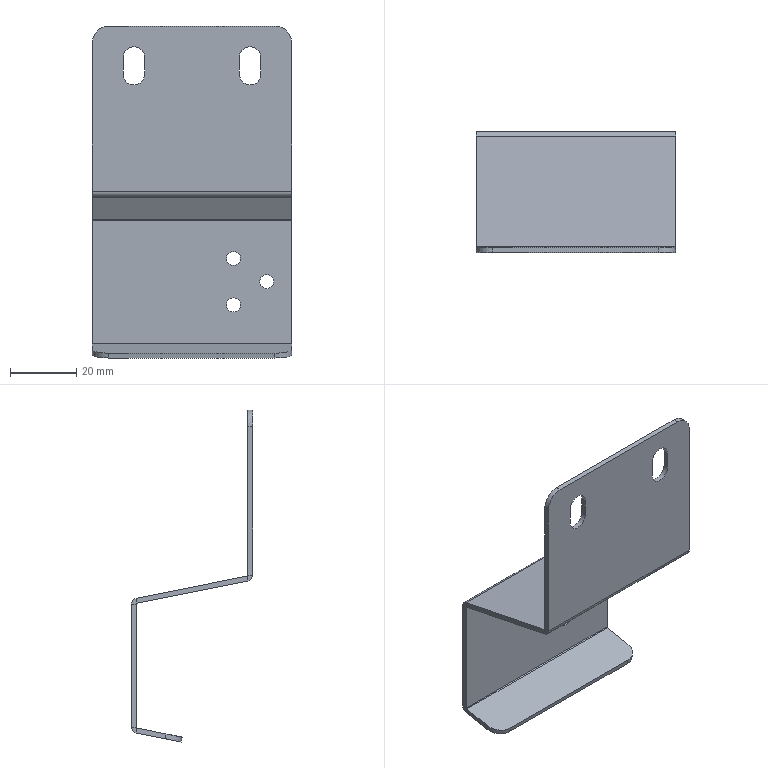Part | SolidWorks | features Cut 1, Fillet 1, FlatPattern 1, HoleWzd 1, SMBaseFlange 1, SheetMetal 1 | 1 solid | 50 faces | box 60 x 36.5 x 100 mm | volume 12211 mm3 | plane 28 | cylinder 22 | commonest cylinder face diameters 4.2 x6 6.5 x6 10 x4 0.6 x3 3.6 x3
STEP:
#1=CARTESIAN_POINT('',(12.5,-1.5,-6.25));
#2=VERTEX_POINT('',#1);
#3=CARTESIAN_POINT('',(15.75,-1.5,-9.5));
#4=VERTEX_POINT('',#3);
#5=CARTESIAN_POINT('',(12.5,-1.5,-9.5));
#6=DIRECTION('',(0.,1.,0.));
#7=DIRECTION('',(0.,0.,1.));
#8=AXIS2_PLACEMENT_3D('',#5,#6,#7);
#9=CIRCLE('',#8,3.25);
#10=EDGE_CURVE('',#2,#4,#9,.T.);
#11=ORIENTED_EDGE('',*,*,#10,.F.);
#12=CARTESIAN_POINT('',(12.5,0.,-6.25));
#13=VERTEX_POINT('',#12);
#14=CARTESIAN_POINT('',(12.5,-10.,-6.25));
#15=DIRECTION('',(0.,1.,0.));
#16=VECTOR('',#15,1000.);
#17=LINE('',#14,#16);
#18=EDGE_CURVE('',#2,#13,#17,.T.);
#19=ORIENTED_EDGE('',*,*,#18,.T.);
#20=CARTESIAN_POINT('',(15.75,0.,-9.5));
#21=VERTEX_POINT('',#20);
#22=CARTESIAN_POINT('',(12.5,0.,-9.5));
#23=DIRECTION('',(0.,1.,0.));
#24=DIRECTION('',(0.,0.,1.));
#25=AXIS2_PLACEMENT_3D('',#22,#23,#24);
#26=CIRCLE('',#25,3.25);
#27=EDGE_CURVE('',#13,#21,#26,.T.);
#28=ORIENTED_EDGE('',*,*,#27,.T.);
#29=CARTESIAN_POINT('',(15.75,-10.,-9.5));
#30=DIRECTION('',(0.,1.,0.));
#31=VECTOR('',#30,1000.);
#32=LINE('',#29,#31);
#33=EDGE_CURVE('',#4,#21,#32,.T.);
#34=ORIENTED_EDGE('',*,*,#33,.F.);
#35=EDGE_LOOP('',(#11,#19,#28,#34));
#36=FACE_OUTER_BOUND('',#35,.T.);
#37=CARTESIAN_POINT('',(12.5,-10.,-9.5));
#38=DIRECTION('',(0.,1.,0.));
#39=DIRECTION('',(0.,0.,1.));
#40=AXIS2_PLACEMENT_3D('',#37,#38,#39);
#41=CYLINDRICAL_SURFACE('',#40,3.25);
#42=ADVANCED_FACE('',(#36),#41,.F.);
#43=CARTESIAN_POINT('',(47.5,-1.5,-6.25));
#44=VERTEX_POINT('',#43);
#45=CARTESIAN_POINT('',(50.75,-1.5,-9.5));
#46=VERTEX_POINT('',#45);
#47=CARTESIAN_POINT('',(47.5,-1.5,-9.5));
#48=DIRECTION('',(0.,1.,0.));
#49=DIRECTION('',(0.,0.,1.));
#50=AXIS2_PLACEMENT_3D('',#47,#48,#49);
#51=CIRCLE('',#50,3.25);
#52=EDGE_CURVE('',#44,#46,#51,.T.);
#53=ORIENTED_EDGE('',*,*,#52,.F.);
#54=CARTESIAN_POINT('',(47.5,0.,-6.25));
#55=VERTEX_POINT('',#54);
#56=CARTESIAN_POINT('',(47.5,-10.,-6.25));
#57=DIRECTION('',(0.,1.,0.));
#58=VECTOR('',#57,1000.);
#59=LINE('',#56,#58);
#60=EDGE_CURVE('',#44,#55,#59,.T.);
#61=ORIENTED_EDGE('',*,*,#60,.T.);
#62=CARTESIAN_POINT('',(50.75,0.,-9.5));
#63=VERTEX_POINT('',#62);
#64=CARTESIAN_POINT('',(47.5,0.,-9.5));
#65=DIRECTION('',(0.,1.,0.));
#66=DIRECTION('',(0.,0.,1.));
#67=AXIS2_PLACEMENT_3D('',#64,#65,#66);
#68=CIRCLE('',#67,3.25);
#69=EDGE_CURVE('',#55,#63,#68,.T.);
#70=ORIENTED_EDGE('',*,*,#69,.T.);
#71=CARTESIAN_POINT('',(50.75,-10.,-9.5));
#72=DIRECTION('',(0.,1.,0.));
#73=VECTOR('',#72,1000.);
#74=LINE('',#71,#73);
#75=EDGE_CURVE('',#46,#63,#74,.T.);
#76=ORIENTED_EDGE('',*,*,#75,.F.);
#77=EDGE_LOOP('',(#53,#61,#70,#76));
#78=FACE_OUTER_BOUND('',#77,.T.);
#79=CARTESIAN_POINT('',(47.5,-10.,-9.5));
#80=DIRECTION('',(0.,1.,0.));
#81=DIRECTION('',(0.,0.,1.));
#82=AXIS2_PLACEMENT_3D('',#79,#80,#81);
#83=CYLINDRICAL_SURFACE('',#82,3.25);
#84=ADVANCED_FACE('',(#78),#83,.F.);
#85=CARTESIAN_POINT('',(42.5,33.5,-86.1));
#86=VERTEX_POINT('',#85);
#87=CARTESIAN_POINT('',(42.5,33.5,-81.9));
#88=VERTEX_POINT('',#87);
#89=CARTESIAN_POINT('',(42.5,33.5,-84.));
#90=DIRECTION('',(0.,1.,0.));
#91=DIRECTION('',(0.,0.,1.));
#92=AXIS2_PLACEMENT_3D('',#89,#90,#91);
#93=CIRCLE('',#92,2.1);
#94=EDGE_CURVE('',#86,#88,#93,.T.);
#95=ORIENTED_EDGE('',*,*,#94,.F.);
#96=CARTESIAN_POINT('',(42.5,35.,-86.1));
#97=VERTEX_POINT('',#96);
#98=CARTESIAN_POINT('',(42.5,35.,-86.1));
#99=DIRECTION('',(0.,1.,0.));
#100=VECTOR('',#99,1000.);
#101=LINE('',#98,#100);
#102=EDGE_CURVE('',#86,#97,#101,.T.);
#103=ORIENTED_EDGE('',*,*,#102,.T.);
#104=CARTESIAN_POINT('',(42.5,35.,-81.9));
#105=VERTEX_POINT('',#104);
#106=CARTESIAN_POINT('',(42.5,35.,-84.));
#107=DIRECTION('',(0.,1.,0.));
#108=DIRECTION('',(0.,0.,1.));
#109=AXIS2_PLACEMENT_3D('',#106,#107,#108);
#110=CIRCLE('',#109,2.1);
#111=EDGE_CURVE('',#97,#105,#110,.T.);
#112=ORIENTED_EDGE('',*,*,#111,.T.);
#113=CARTESIAN_POINT('',(42.5,35.,-81.9));
#114=DIRECTION('',(0.,1.,0.));
#115=VECTOR('',#114,1000.);
#116=LINE('',#113,#115);
#117=EDGE_CURVE('',#88,#105,#116,.T.);
#118=ORIENTED_EDGE('',*,*,#117,.F.);
#119=EDGE_LOOP('',(#95,#103,#112,#118));
#120=FACE_OUTER_BOUND('',#119,.T.);
#121=CARTESIAN_POINT('',(42.5,35.,-84.));
#122=DIRECTION('',(0.,1.,0.));
#123=DIRECTION('',(0.,0.,1.));
#124=AXIS2_PLACEMENT_3D('',#121,#122,#123);
#125=CYLINDRICAL_SURFACE('',#124,2.1);
#126=ADVANCED_FACE('',(#120),#125,.F.);
#127=CARTESIAN_POINT('',(42.5,33.5,-72.1));
#128=VERTEX_POINT('',#127);
#129=CARTESIAN_POINT('',(42.5,33.5,-67.9));
#130=VERTEX_POINT('',#129);
#131=CARTESIAN_POINT('',(42.5,33.5,-70.));
#132=DIRECTION('',(0.,1.,0.));
#133=DIRECTION('',(0.,0.,1.));
#134=AXIS2_PLACEMENT_3D('',#131,#132,#133);
#135=CIRCLE('',#134,2.1);
#136=EDGE_CURVE('',#128,#130,#135,.T.);
#137=ORIENTED_EDGE('',*,*,#136,.F.);
#138=CARTESIAN_POINT('',(42.5,35.,-72.1));
#139=VERTEX_POINT('',#138);
#140=CARTESIAN_POINT('',(42.5,35.,-72.1));
#141=DIRECTION('',(0.,1.,0.));
#142=VECTOR('',#141,1000.);
#143=LINE('',#140,#142);
#144=EDGE_CURVE('',#128,#139,#143,.T.);
#145=ORIENTED_EDGE('',*,*,#144,.T.);
#146=CARTESIAN_POINT('',(42.5,35.,-67.9));
#147=VERTEX_POINT('',#146);
#148=CARTESIAN_POINT('',(42.5,35.,-70.));
#149=DIRECTION('',(0.,1.,0.));
#150=DIRECTION('',(0.,0.,1.));
#151=AXIS2_PLACEMENT_3D('',#148,#149,#150);
#152=CIRCLE('',#151,2.1);
#153=EDGE_CURVE('',#139,#147,#152,.T.);
#154=ORIENTED_EDGE('',*,*,#153,.T.);
#155=CARTESIAN_POINT('',(42.5,35.,-67.9));
#156=DIRECTION('',(0.,1.,0.));
#157=VECTOR('',#156,1000.);
#158=LINE('',#155,#157);
#159=EDGE_CURVE('',#130,#147,#158,.T.);
#160=ORIENTED_EDGE('',*,*,#159,.F.);
#161=EDGE_LOOP('',(#137,#145,#154,#160));
#162=FACE_OUTER_BOUND('',#161,.T.);
#163=CARTESIAN_POINT('',(42.5,35.,-70.));
#164=DIRECTION('',(0.,1.,0.));
#165=DIRECTION('',(0.,0.,1.));
#166=AXIS2_PLACEMENT_3D('',#163,#164,#165);
#167=CYLINDRICAL_SURFACE('',#166,2.1);
#168=ADVANCED_FACE('',(#162),#167,.F.);
#169=CARTESIAN_POINT('',(52.5,33.5,-79.1));
#170=VERTEX_POINT('',#169);
#171=CARTESIAN_POINT('',(52.5,33.5,-74.9));
#172=VERTEX_POINT('',#171);
#173=CARTESIAN_POINT('',(52.5,33.5,-77.));
#174=DIRECTION('',(0.,1.,0.));
#175=DIRECTION('',(0.,0.,1.));
#176=AXIS2_PLACEMENT_3D('',#173,#174,#175);
#177=CIRCLE('',#176,2.1);
#178=EDGE_CURVE('',#170,#172,#177,.T.);
#179=ORIENTED_EDGE('',*,*,#178,.F.);
#180=CARTESIAN_POINT('',(52.5,35.,-79.1));
#181=VERTEX_POINT('',#180);
#182=CARTESIAN_POINT('',(52.5,35.,-79.1));
#183=DIRECTION('',(0.,1.,0.));
#184=VECTOR('',#183,1000.);
#185=LINE('',#182,#184);
#186=EDGE_CURVE('',#170,#181,#185,.T.);
#187=ORIENTED_EDGE('',*,*,#186,.T.);
#188=CARTESIAN_POINT('',(52.5,35.,-74.9));
#189=VERTEX_POINT('',#188);
#190=CARTESIAN_POINT('',(52.5,35.,-77.));
#191=DIRECTION('',(0.,1.,0.));
#192=DIRECTION('',(0.,0.,1.));
#193=AXIS2_PLACEMENT_3D('',#190,#191,#192);
#194=CIRCLE('',#193,2.1);
#195=EDGE_CURVE('',#181,#189,#194,.T.);
#196=ORIENTED_EDGE('',*,*,#195,.T.);
#197=CARTESIAN_POINT('',(52.5,35.,-74.9));
#198=DIRECTION('',(0.,1.,0.));
#199=VECTOR('',#198,1000.);
#200=LINE('',#197,#199);
#201=EDGE_CURVE('',#172,#189,#200,.T.);
#202=ORIENTED_EDGE('',*,*,#201,.F.);
#203=EDGE_LOOP('',(#179,#187,#196,#202));
#204=FACE_OUTER_BOUND('',#203,.T.);
#205=CARTESIAN_POINT('',(52.5,35.,-77.));
#206=DIRECTION('',(0.,1.,0.));
#207=DIRECTION('',(0.,0.,1.));
#208=AXIS2_PLACEMENT_3D('',#205,#206,#207);
#209=CYLINDRICAL_SURFACE('',#208,2.1);
#210=ADVANCED_FACE('',(#204),#209,.F.);
#211=CARTESIAN_POINT('',(60.,0.2412,-50.048));
#212=VERTEX_POINT('',#211);
#213=CARTESIAN_POINT('',(60.,-0.05301,-51.519));
#214=VERTEX_POINT('',#213);
#215=CARTESIAN_POINT('',(60.,0.2412,-50.048));
#216=DIRECTION('',(0.,-0.1961,-0.9806));
#217=VECTOR('',#216,1000.);
#218=LINE('',#215,#217);
#219=EDGE_CURVE('',#212,#214,#218,.T.);
#220=ORIENTED_EDGE('',*,*,#219,.F.);
#221=CARTESIAN_POINT('',(60.,0.,-49.754));
#222=VERTEX_POINT('',#221);
#223=CARTESIAN_POINT('',(60.,0.3,-49.754));
#224=DIRECTION('',(1.,0.,0.));
#225=DIRECTION('',(0.,0.,1.));
#226=AXIS2_PLACEMENT_3D('',#223,#224,#225);
#227=CIRCLE('',#226,0.3);
#228=EDGE_CURVE('',#222,#212,#227,.T.);
#229=ORIENTED_EDGE('',*,*,#228,.F.);
#230=CARTESIAN_POINT('',(60.,-1.5,-49.754));
#231=VERTEX_POINT('',#230);
#232=CARTESIAN_POINT('',(60.,-1.5,-49.754));
#233=DIRECTION('',(0.,1.,0.));
#234=VECTOR('',#233,1000.);
#235=LINE('',#232,#234);
#236=EDGE_CURVE('',#231,#222,#235,.T.);
#237=ORIENTED_EDGE('',*,*,#236,.F.);
#238=CARTESIAN_POINT('',(60.,0.3,-49.754));
#239=DIRECTION('',(1.,0.,0.));
#240=DIRECTION('',(0.,0.,-1.));
#241=AXIS2_PLACEMENT_3D('',#238,#239,#240);
#242=CIRCLE('',#241,1.8);
#243=EDGE_CURVE('',#231,#214,#242,.T.);
#244=ORIENTED_EDGE('',*,*,#243,.T.);
#245=EDGE_LOOP('',(#220,#229,#237,#244));
#246=FACE_OUTER_BOUND('',#245,.T.);
#247=CARTESIAN_POINT('',(60.,0.2412,-50.048));
#248=DIRECTION('',(1.,0.,0.));
#249=DIRECTION('',(0.,0.,-1.));
#250=AXIS2_PLACEMENT_3D('',#247,#248,#249);
#251=PLANE('',#250);
#252=ADVANCED_FACE('',(#246),#251,.T.);
#253=CARTESIAN_POINT('',(60.,33.553,-56.711));
#254=VERTEX_POINT('',#253);
#255=CARTESIAN_POINT('',(60.,0.,-50.));
#256=DIRECTION('',(0.,0.9806,-0.1961));
#257=VECTOR('',#256,1000.);
#258=LINE('',#255,#257);
#259=EDGE_CURVE('',#212,#254,#258,.T.);
#260=ORIENTED_EDGE('',*,*,#259,.F.);
#261=ORIENTED_EDGE('',*,*,#219,.T.);
#262=CARTESIAN_POINT('',(60.,33.259,-58.181));
#263=VERTEX_POINT('',#262);
#264=CARTESIAN_POINT('',(60.,-0.2942,-51.471));
#265=DIRECTION('',(0.,0.9806,-0.1961));
#266=VECTOR('',#265,1000.);
#267=LINE('',#264,#266);
#268=EDGE_CURVE('',#214,#263,#267,.T.);
#269=ORIENTED_EDGE('',*,*,#268,.T.);
#270=CARTESIAN_POINT('',(60.,33.259,-58.181));
#271=DIRECTION('',(0.,0.1961,0.9806));
#272=VECTOR('',#271,1000.);
#273=LINE('',#270,#272);
#274=EDGE_CURVE('',#263,#254,#273,.T.);
#275=ORIENTED_EDGE('',*,*,#274,.T.);
#276=EDGE_LOOP('',(#260,#261,#269,#275));
#277=FACE_OUTER_BOUND('',#276,.T.);
#278=CARTESIAN_POINT('',(60.,-1.5,-49.754));
#279=DIRECTION('',(1.,0.,0.));
#280=DIRECTION('',(0.,0.,-1.));
#281=AXIS2_PLACEMENT_3D('',#278,#279,#280);
#282=PLANE('',#281);
#283=ADVANCED_FACE('',(#277),#282,.T.);
#284=CARTESIAN_POINT('',(0.,0.,-49.754));
#285=VERTEX_POINT('',#284);
#286=CARTESIAN_POINT('',(0.,-1.5,-49.754));
#287=VERTEX_POINT('',#286);
#288=CARTESIAN_POINT('',(0.,0.,-49.754));
#289=DIRECTION('',(0.,-1.,0.));
#290=VECTOR('',#289,1000.);
#291=LINE('',#288,#290);
#292=EDGE_CURVE('',#285,#287,#291,.T.);
#293=ORIENTED_EDGE('',*,*,#292,.F.);
#294=CARTESIAN_POINT('',(0.,0.2412,-50.048));
#295=VERTEX_POINT('',#294);
#296=CARTESIAN_POINT('',(0.,0.3,-49.754));
#297=DIRECTION('',(1.,0.,0.));
#298=DIRECTION('',(0.,0.,1.));
#299=AXIS2_PLACEMENT_3D('',#296,#297,#298);
#300=CIRCLE('',#299,0.3);
#301=EDGE_CURVE('',#285,#295,#300,.T.);
#302=ORIENTED_EDGE('',*,*,#301,.T.);
#303=CARTESIAN_POINT('',(0.,-0.05301,-51.519));
#304=VERTEX_POINT('',#303);
#305=CARTESIAN_POINT('',(0.,-0.05301,-51.519));
#306=DIRECTION('',(0.,0.1961,0.9806));
#307=VECTOR('',#306,1000.);
#308=LINE('',#305,#307);
#309=EDGE_CURVE('',#304,#295,#308,.T.);
#310=ORIENTED_EDGE('',*,*,#309,.F.);
#311=CARTESIAN_POINT('',(0.,0.3,-49.754));
#312=DIRECTION('',(1.,0.,0.));
#313=DIRECTION('',(0.,0.,-1.));
#314=AXIS2_PLACEMENT_3D('',#311,#312,#313);
#315=CIRCLE('',#314,1.8);
#316=EDGE_CURVE('',#287,#304,#315,.T.);
#317=ORIENTED_EDGE('',*,*,#316,.F.);
#318=EDGE_LOOP('',(#293,#302,#310,#317));
#319=FACE_OUTER_BOUND('',#318,.T.);
#320=CARTESIAN_POINT('',(0.,0.,-49.754));
#321=DIRECTION('',(-1.,0.,0.));
#322=DIRECTION('',(0.,0.,1.));
#323=AXIS2_PLACEMENT_3D('',#320,#321,#322);
#324=PLANE('',#323);
#325=ADVANCED_FACE('',(#319),#324,.T.);
#326=CARTESIAN_POINT('',(0.,-1.5,-5.));
#327=VERTEX_POINT('',#326);
#328=CARTESIAN_POINT('',(0.,-1.5,0.));
#329=DIRECTION('',(0.,0.,-1.));
#330=VECTOR('',#329,1000.);
#331=LINE('',#328,#330);
#332=EDGE_CURVE('',#327,#287,#331,.T.);
#333=ORIENTED_EDGE('',*,*,#332,.F.);
#334=CARTESIAN_POINT('',(0.,0.,-5.));
#335=VERTEX_POINT('',#334);
#336=CARTESIAN_POINT('',(0.,-0.05301,-5.));
#337=DIRECTION('',(0.,1.,0.));
#338=VECTOR('',#337,1000.);
#339=LINE('',#336,#338);
#340=EDGE_CURVE('',#327,#335,#339,.T.);
#341=ORIENTED_EDGE('',*,*,#340,.T.);
#342=CARTESIAN_POINT('',(0.,0.,0.));
#343=DIRECTION('',(0.,0.,-1.));
#344=VECTOR('',#343,1000.);
#345=LINE('',#342,#344);
#346=EDGE_CURVE('',#335,#285,#345,.T.);
#347=ORIENTED_EDGE('',*,*,#346,.T.);
#348=ORIENTED_EDGE('',*,*,#292,.T.);
#349=EDGE_LOOP('',(#333,#341,#347,#348));
#350=FACE_OUTER_BOUND('',#349,.T.);
#351=CARTESIAN_POINT('',(0.,-0.05301,-51.519));
#352=DIRECTION('',(-1.,0.,0.));
#353=DIRECTION('',(0.,0.,1.));
#354=AXIS2_PLACEMENT_3D('',#351,#352,#353);
#355=PLANE('',#354);
#356=ADVANCED_FACE('',(#350),#355,.T.);
#357=CARTESIAN_POINT('',(60.,35.,-58.476));
#358=VERTEX_POINT('',#357);
#359=CARTESIAN_POINT('',(60.,33.5,-58.476));
#360=VERTEX_POINT('',#359);
#361=CARTESIAN_POINT('',(60.,35.,-58.476));
#362=DIRECTION('',(0.,-1.,0.));
#363=VECTOR('',#362,1000.);
#364=LINE('',#361,#363);
#365=EDGE_CURVE('',#358,#360,#364,.T.);
#366=ORIENTED_EDGE('',*,*,#365,.F.);
#367=CARTESIAN_POINT('',(60.,33.2,-58.476));
#368=DIRECTION('',(-1.,0.,0.));
#369=DIRECTION('',(0.,0.,-1.));
#370=AXIS2_PLACEMENT_3D('',#367,#368,#369);
#371=CIRCLE('',#370,1.8);
#372=EDGE_CURVE('',#254,#358,#371,.T.);
#373=ORIENTED_EDGE('',*,*,#372,.F.);
#374=ORIENTED_EDGE('',*,*,#274,.F.);
#375=CARTESIAN_POINT('',(60.,33.2,-58.476));
#376=DIRECTION('',(-1.,0.,0.));
#377=DIRECTION('',(0.,0.,-1.));
#378=AXIS2_PLACEMENT_3D('',#375,#376,#377);
#379=CIRCLE('',#378,0.3);
#380=EDGE_CURVE('',#263,#360,#379,.T.);
#381=ORIENTED_EDGE('',*,*,#380,.T.);
#382=EDGE_LOOP('',(#366,#373,#374,#381));
#383=FACE_OUTER_BOUND('',#382,.T.);
#384=CARTESIAN_POINT('',(60.,35.,-58.476));
#385=DIRECTION('',(1.,0.,0.));
#386=DIRECTION('',(0.,0.,-1.));
#387=AXIS2_PLACEMENT_3D('',#384,#385,#386);
#388=PLANE('',#387);
#389=ADVANCED_FACE('',(#383),#388,.T.);
#390=CARTESIAN_POINT('',(60.,35.,-95.524));
#391=VERTEX_POINT('',#390);
#392=CARTESIAN_POINT('',(60.,35.,-57.));
#393=DIRECTION('',(0.,0.,-1.));
#394=VECTOR('',#393,1000.);
#395=LINE('',#392,#394);
#396=EDGE_CURVE('',#358,#391,#395,.T.);
#397=ORIENTED_EDGE('',*,*,#396,.F.);
#398=ORIENTED_EDGE('',*,*,#365,.T.);
#399=CARTESIAN_POINT('',(60.,33.5,-95.524));
#400=VERTEX_POINT('',#399);
#401=CARTESIAN_POINT('',(60.,33.5,-57.));
#402=DIRECTION('',(0.,0.,-1.));
#403=VECTOR('',#402,1000.);
#404=LINE('',#401,#403);
#405=EDGE_CURVE('',#360,#400,#404,.T.);
#406=ORIENTED_EDGE('',*,*,#405,.T.);
#407=CARTESIAN_POINT('',(60.,33.5,-95.524));
#408=DIRECTION('',(0.,1.,0.));
#409=VECTOR('',#408,1000.);
#410=LINE('',#407,#409);
#411=EDGE_CURVE('',#400,#391,#410,.T.);
#412=ORIENTED_EDGE('',*,*,#411,.T.);
#413=EDGE_LOOP('',(#397,#398,#406,#412));
#414=FACE_OUTER_BOUND('',#413,.T.);
#415=CARTESIAN_POINT('',(60.,33.259,-58.181));
#416=DIRECTION('',(1.,0.,0.));
#417=DIRECTION('',(0.,0.,-1.));
#418=AXIS2_PLACEMENT_3D('',#415,#416,#417);
#419=PLANE('',#418);
#420=ADVANCED_FACE('',(#414),#419,.T.);
#421=CARTESIAN_POINT('',(0.,33.553,-56.711));
#422=VERTEX_POINT('',#421);
#423=CARTESIAN_POINT('',(0.,33.259,-58.181));
#424=VERTEX_POINT('',#423);
#425=CARTESIAN_POINT('',(0.,33.553,-56.711));
#426=DIRECTION('',(0.,-0.1961,-0.9806));
#427=VECTOR('',#426,1000.);
#428=LINE('',#425,#427);
#429=EDGE_CURVE('',#422,#424,#428,.T.);
#430=ORIENTED_EDGE('',*,*,#429,.F.);
#431=CARTESIAN_POINT('',(0.,35.,-58.476));
#432=VERTEX_POINT('',#431);
#433=CARTESIAN_POINT('',(0.,33.2,-58.476));
#434=DIRECTION('',(-1.,0.,0.));
#435=DIRECTION('',(0.,0.,-1.));
#436=AXIS2_PLACEMENT_3D('',#433,#434,#435);
#437=CIRCLE('',#436,1.8);
#438=EDGE_CURVE('',#422,#432,#437,.T.);
#439=ORIENTED_EDGE('',*,*,#438,.T.);
#440=CARTESIAN_POINT('',(0.,33.5,-58.476));
#441=VERTEX_POINT('',#440);
#442=CARTESIAN_POINT('',(0.,33.5,-58.476));
#443=DIRECTION('',(0.,1.,0.));
#444=VECTOR('',#443,1000.);
#445=LINE('',#442,#444);
#446=EDGE_CURVE('',#441,#432,#445,.T.);
#447=ORIENTED_EDGE('',*,*,#446,.F.);
#448=CARTESIAN_POINT('',(0.,33.2,-58.476));
#449=DIRECTION('',(-1.,0.,0.));
#450=DIRECTION('',(0.,0.,-1.));
#451=AXIS2_PLACEMENT_3D('',#448,#449,#450);
#452=CIRCLE('',#451,0.3);
#453=EDGE_CURVE('',#424,#441,#452,.T.);
#454=ORIENTED_EDGE('',*,*,#453,.F.);
#455=EDGE_LOOP('',(#430,#439,#447,#454));
#456=FACE_OUTER_BOUND('',#455,.T.);
#457=CARTESIAN_POINT('',(0.,33.553,-56.711));
#458=DIRECTION('',(-1.,0.,0.));
#459=DIRECTION('',(0.,0.,1.));
#460=AXIS2_PLACEMENT_3D('',#457,#458,#459);
#461=PLANE('',#460);
#462=ADVANCED_FACE('',(#456),#461,.T.);
#463=CARTESIAN_POINT('',(0.,0.,-50.));
#464=DIRECTION('',(0.,0.9806,-0.1961));
#465=VECTOR('',#464,1000.);
#466=LINE('',#463,#465);
#467=EDGE_CURVE('',#295,#422,#466,.T.);
#468=ORIENTED_EDGE('',*,*,#467,.T.);
#469=ORIENTED_EDGE('',*,*,#429,.T.);
#470=CARTESIAN_POINT('',(0.,-0.2942,-51.471));
#471=DIRECTION('',(0.,0.9806,-0.1961));
#472=VECTOR('',#471,1000.);
#473=LINE('',#470,#472);
#474=EDGE_CURVE('',#304,#424,#473,.T.);
#475=ORIENTED_EDGE('',*,*,#474,.F.);
#476=ORIENTED_EDGE('',*,*,#309,.T.);
#477=EDGE_LOOP('',(#468,#469,#475,#476));
#478=FACE_OUTER_BOUND('',#477,.T.);
#479=CARTESIAN_POINT('',(0.,33.5,-58.476));
#480=DIRECTION('',(-1.,0.,0.));
#481=DIRECTION('',(0.,0.,1.));
#482=AXIS2_PLACEMENT_3D('',#479,#480,#481);
#483=PLANE('',#482);
#484=ADVANCED_FACE('',(#478),#483,.T.);
#485=CARTESIAN_POINT('',(60.,33.553,-97.289));
#486=VERTEX_POINT('',#485);
#487=CARTESIAN_POINT('',(60.,33.259,-95.819));
#488=VERTEX_POINT('',#487);
#489=CARTESIAN_POINT('',(60.,33.553,-97.289));
#490=DIRECTION('',(0.,-0.1961,0.9806));
#491=VECTOR('',#490,1000.);
#492=LINE('',#489,#491);
#493=EDGE_CURVE('',#486,#488,#492,.T.);
#494=ORIENTED_EDGE('',*,*,#493,.F.);
#495=CARTESIAN_POINT('',(60.,33.2,-95.524));
#496=DIRECTION('',(-1.,0.,0.));
#497=DIRECTION('',(0.,0.,-1.));
#498=AXIS2_PLACEMENT_3D('',#495,#496,#497);
#499=CIRCLE('',#498,1.8);
#500=EDGE_CURVE('',#391,#486,#499,.T.);
#501=ORIENTED_EDGE('',*,*,#500,.F.);
#502=ORIENTED_EDGE('',*,*,#411,.F.);
#503=CARTESIAN_POINT('',(60.,33.2,-95.524));
#504=DIRECTION('',(-1.,0.,0.));
#505=DIRECTION('',(0.,0.,-1.));
#506=AXIS2_PLACEMENT_3D('',#503,#504,#505);
#507=CIRCLE('',#506,0.3);
#508=EDGE_CURVE('',#400,#488,#507,.T.);
#509=ORIENTED_EDGE('',*,*,#508,.T.);
#510=EDGE_LOOP('',(#494,#501,#502,#509));
#511=FACE_OUTER_BOUND('',#510,.T.);
#512=CARTESIAN_POINT('',(60.,33.553,-97.289));
#513=DIRECTION('',(1.,0.,0.));
#514=DIRECTION('',(0.,0.,-1.));
#515=AXIS2_PLACEMENT_3D('',#512,#513,#514);
#516=PLANE('',#515);
#517=ADVANCED_FACE('',(#511),#516,.T.);
#518=CARTESIAN_POINT('',(60.,24.609,-97.549));
#519=VERTEX_POINT('',#518);
#520=CARTESIAN_POINT('',(60.,34.706,-95.529));
#521=DIRECTION('',(0.,-0.9806,-0.1961));
#522=VECTOR('',#521,1000.);
#523=LINE('',#520,#522);
#524=EDGE_CURVE('',#488,#519,#523,.T.);
#525=ORIENTED_EDGE('',*,*,#524,.T.);
#526=CARTESIAN_POINT('',(60.,24.903,-99.019));
#527=VERTEX_POINT('',#526);
#528=CARTESIAN_POINT('',(60.,24.561,-97.312));
#529=DIRECTION('',(0.,0.1961,-0.9806));
#530=VECTOR('',#529,1000.);
#531=LINE('',#528,#530);
#532=EDGE_CURVE('',#519,#527,#531,.T.);
#533=ORIENTED_EDGE('',*,*,#532,.T.);
#534=CARTESIAN_POINT('',(60.,35.,-97.));
#535=DIRECTION('',(0.,-0.9806,-0.1961));
#536=VECTOR('',#535,1000.);
#537=LINE('',#534,#536);
#538=EDGE_CURVE('',#486,#527,#537,.T.);
#539=ORIENTED_EDGE('',*,*,#538,.F.);
#540=ORIENTED_EDGE('',*,*,#493,.T.);
#541=EDGE_LOOP('',(#525,#533,#539,#540));
#542=FACE_OUTER_BOUND('',#541,.T.);
#543=CARTESIAN_POINT('',(60.,33.5,-95.524));
#544=DIRECTION('',(1.,0.,0.));
#545=DIRECTION('',(0.,0.,-1.));
#546=AXIS2_PLACEMENT_3D('',#543,#544,#545);
#547=PLANE('',#546);
#548=ADVANCED_FACE('',(#542),#547,.T.);
#549=CARTESIAN_POINT('',(0.,35.,-95.524));
#550=VERTEX_POINT('',#549);
#551=CARTESIAN_POINT('',(0.,33.5,-95.524));
#552=VERTEX_POINT('',#551);
#553=CARTESIAN_POINT('',(0.,35.,-95.524));
#554=DIRECTION('',(0.,-1.,0.));
#555=VECTOR('',#554,1000.);
#556=LINE('',#553,#555);
#557=EDGE_CURVE('',#550,#552,#556,.T.);
#558=ORIENTED_EDGE('',*,*,#557,.F.);
#559=CARTESIAN_POINT('',(0.,33.553,-97.289));
#560=VERTEX_POINT('',#559);
#561=CARTESIAN_POINT('',(0.,33.2,-95.524));
#562=DIRECTION('',(-1.,0.,0.));
#563=DIRECTION('',(0.,0.,-1.));
#564=AXIS2_PLACEMENT_3D('',#561,#562,#563);
#565=CIRCLE('',#564,1.8);
#566=EDGE_CURVE('',#550,#560,#565,.T.);
#567=ORIENTED_EDGE('',*,*,#566,.T.);
#568=CARTESIAN_POINT('',(0.,33.259,-95.819));
#569=VERTEX_POINT('',#568);
#570=CARTESIAN_POINT('',(0.,33.259,-95.819));
#571=DIRECTION('',(0.,0.1961,-0.9806));
#572=VECTOR('',#571,1000.);
#573=LINE('',#570,#572);
#574=EDGE_CURVE('',#569,#560,#573,.T.);
#575=ORIENTED_EDGE('',*,*,#574,.F.);
#576=CARTESIAN_POINT('',(0.,33.2,-95.524));
#577=DIRECTION('',(-1.,0.,0.));
#578=DIRECTION('',(0.,0.,-1.));
#579=AXIS2_PLACEMENT_3D('',#576,#577,#578);
#580=CIRCLE('',#579,0.3);
#581=EDGE_CURVE('',#552,#569,#580,.T.);
#582=ORIENTED_EDGE('',*,*,#581,.F.);
#583=EDGE_LOOP('',(#558,#567,#575,#582));
#584=FACE_OUTER_BOUND('',#583,.T.);
#585=CARTESIAN_POINT('',(0.,35.,-95.524));
#586=DIRECTION('',(-1.,0.,0.));
#587=DIRECTION('',(0.,0.,1.));
#588=AXIS2_PLACEMENT_3D('',#585,#586,#587);
#589=PLANE('',#588);
#590=ADVANCED_FACE('',(#584),#589,.T.);
#591=CARTESIAN_POINT('',(0.,35.,-57.));
#592=DIRECTION('',(0.,0.,-1.));
#593=VECTOR('',#592,1000.);
#594=LINE('',#591,#593);
#595=EDGE_CURVE('',#432,#550,#594,.T.);
#596=ORIENTED_EDGE('',*,*,#595,.T.);
#597=ORIENTED_EDGE('',*,*,#557,.T.);
#598=CARTESIAN_POINT('',(0.,33.5,-57.));
#599=DIRECTION('',(0.,0.,-1.));
#600=VECTOR('',#599,1000.);
#601=LINE('',#598,#600);
#602=EDGE_CURVE('',#441,#552,#601,.T.);
#603=ORIENTED_EDGE('',*,*,#602,.F.);
#604=ORIENTED_EDGE('',*,*,#446,.T.);
#605=EDGE_LOOP('',(#596,#597,#603,#604));
#606=FACE_OUTER_BOUND('',#605,.T.);
#607=CARTESIAN_POINT('',(0.,33.259,-95.819));
#608=DIRECTION('',(-1.,0.,0.));
#609=DIRECTION('',(0.,0.,1.));
#610=AXIS2_PLACEMENT_3D('',#607,#608,#609);
#611=PLANE('',#610);
#612=ADVANCED_FACE('',(#606),#611,.T.);
#613=CARTESIAN_POINT('',(0.,24.609,-97.549));
#614=VERTEX_POINT('',#613);
#615=CARTESIAN_POINT('',(0.,34.706,-95.529));
#616=DIRECTION('',(0.,-0.9806,-0.1961));
#617=VECTOR('',#616,1000.);
#618=LINE('',#615,#617);
#619=EDGE_CURVE('',#569,#614,#618,.T.);
#620=ORIENTED_EDGE('',*,*,#619,.T.);
#621=CARTESIAN_POINT('',(5.,19.706,-98.529));
#622=VERTEX_POINT('',#621);
#623=CARTESIAN_POINT('',(5.,24.609,-97.549));
#624=DIRECTION('',(0.,-0.1961,0.9806));
#625=DIRECTION('',(0.,0.9806,0.1961));
#626=AXIS2_PLACEMENT_3D('',#623,#624,#625);
#627=CIRCLE('',#626,5.);
#628=EDGE_CURVE('',#614,#622,#627,.T.);
#629=ORIENTED_EDGE('',*,*,#628,.T.);
#630=CARTESIAN_POINT('',(55.,19.706,-98.529));
#631=VERTEX_POINT('',#630);
#632=CARTESIAN_POINT('',(60.,19.706,-98.529));
#633=DIRECTION('',(-1.,0.,0.));
#634=VECTOR('',#633,1000.);
#635=LINE('',#632,#634);
#636=EDGE_CURVE('',#631,#622,#635,.T.);
#637=ORIENTED_EDGE('',*,*,#636,.F.);
#638=CARTESIAN_POINT('',(55.,24.609,-97.549));
#639=DIRECTION('',(0.,-0.1961,0.9806));
#640=DIRECTION('',(0.,0.9806,0.1961));
#641=AXIS2_PLACEMENT_3D('',#638,#639,#640);
#642=CIRCLE('',#641,5.);
#643=EDGE_CURVE('',#631,#519,#642,.T.);
#644=ORIENTED_EDGE('',*,*,#643,.T.);
#645=ORIENTED_EDGE('',*,*,#524,.F.);
#646=CARTESIAN_POINT('',(60.,33.259,-95.819));
#647=DIRECTION('',(-1.,0.,0.));
#648=VECTOR('',#647,1000.);
#649=LINE('',#646,#648);
#650=EDGE_CURVE('',#488,#569,#649,.T.);
#651=ORIENTED_EDGE('',*,*,#650,.T.);
#652=EDGE_LOOP('',(#620,#629,#637,#644,#645,#651));
#653=FACE_OUTER_BOUND('',#652,.T.);
#654=CARTESIAN_POINT('',(60.,34.706,-95.529));
#655=DIRECTION('',(0.,0.1961,-0.9806));
#656=DIRECTION('',(0.,0.9806,0.1961));
#657=AXIS2_PLACEMENT_3D('',#654,#655,#656);
#658=PLANE('',#657);
#659=ADVANCED_FACE('',(#653),#658,.F.);
#660=ORIENTED_EDGE('',*,*,#636,.T.);
#661=CARTESIAN_POINT('',(5.,20.,-100.));
#662=VERTEX_POINT('',#661);
#663=CARTESIAN_POINT('',(5.,20.,-100.));
#664=DIRECTION('',(0.,0.1961,-0.9806));
#665=VECTOR('',#664,1000.);
#666=LINE('',#663,#665);
#667=EDGE_CURVE('',#622,#662,#666,.T.);
#668=ORIENTED_EDGE('',*,*,#667,.T.);
#669=CARTESIAN_POINT('',(55.,20.,-100.));
#670=VERTEX_POINT('',#669);
#671=CARTESIAN_POINT('',(60.,20.,-100.));
#672=DIRECTION('',(-1.,0.,0.));
#673=VECTOR('',#672,1000.);
#674=LINE('',#671,#673);
#675=EDGE_CURVE('',#670,#662,#674,.T.);
#676=ORIENTED_EDGE('',*,*,#675,.F.);
#677=CARTESIAN_POINT('',(55.,20.,-100.));
#678=DIRECTION('',(0.,-0.1961,0.9806));
#679=VECTOR('',#678,1000.);
#680=LINE('',#677,#679);
#681=EDGE_CURVE('',#670,#631,#680,.T.);
#682=ORIENTED_EDGE('',*,*,#681,.T.);
#683=EDGE_LOOP('',(#660,#668,#676,#682));
#684=FACE_OUTER_BOUND('',#683,.T.);
#685=CARTESIAN_POINT('',(60.,20.,-100.));
#686=DIRECTION('',(0.,-0.9806,-0.1961));
#687=DIRECTION('',(0.,0.1961,-0.9806));
#688=AXIS2_PLACEMENT_3D('',#685,#686,#687);
#689=PLANE('',#688);
#690=ADVANCED_FACE('',(#684),#689,.T.);
#691=ORIENTED_EDGE('',*,*,#675,.T.);
#692=CARTESIAN_POINT('',(0.,24.903,-99.019));
#693=VERTEX_POINT('',#692);
#694=CARTESIAN_POINT('',(5.,24.903,-99.019));
#695=DIRECTION('',(0.,0.1961,-0.9806));
#696=DIRECTION('',(0.,0.9806,0.1961));
#697=AXIS2_PLACEMENT_3D('',#694,#695,#696);
#698=CIRCLE('',#697,5.);
#699=EDGE_CURVE('',#662,#693,#698,.T.);
#700=ORIENTED_EDGE('',*,*,#699,.T.);
#701=CARTESIAN_POINT('',(0.,35.,-97.));
#702=DIRECTION('',(0.,-0.9806,-0.1961));
#703=VECTOR('',#702,1000.);
#704=LINE('',#701,#703);
#705=EDGE_CURVE('',#560,#693,#704,.T.);
#706=ORIENTED_EDGE('',*,*,#705,.F.);
#707=CARTESIAN_POINT('',(60.,33.553,-97.289));
#708=DIRECTION('',(-1.,0.,0.));
#709=VECTOR('',#708,1000.);
#710=LINE('',#707,#709);
#711=EDGE_CURVE('',#486,#560,#710,.T.);
#712=ORIENTED_EDGE('',*,*,#711,.F.);
#713=ORIENTED_EDGE('',*,*,#538,.T.);
#714=CARTESIAN_POINT('',(55.,24.903,-99.019));
#715=DIRECTION('',(0.,0.1961,-0.9806));
#716=DIRECTION('',(0.,0.9806,0.1961));
#717=AXIS2_PLACEMENT_3D('',#714,#715,#716);
#718=CIRCLE('',#717,5.);
#719=EDGE_CURVE('',#527,#670,#718,.T.);
#720=ORIENTED_EDGE('',*,*,#719,.T.);
#721=EDGE_LOOP('',(#691,#700,#706,#712,#713,#720));
#722=FACE_OUTER_BOUND('',#721,.T.);
#723=CARTESIAN_POINT('',(60.,35.,-97.));
#724=DIRECTION('',(0.,0.1961,-0.9806));
#725=DIRECTION('',(0.,0.9806,0.1961));
#726=AXIS2_PLACEMENT_3D('',#723,#724,#725);
#727=PLANE('',#726);
#728=ADVANCED_FACE('',(#722),#727,.T.);
#729=ORIENTED_EDGE('',*,*,#566,.F.);
#730=CARTESIAN_POINT('',(60.,35.,-95.524));
#731=DIRECTION('',(-1.,0.,0.));
#732=VECTOR('',#731,1000.);
#733=LINE('',#730,#732);
#734=EDGE_CURVE('',#391,#550,#733,.T.);
#735=ORIENTED_EDGE('',*,*,#734,.F.);
#736=ORIENTED_EDGE('',*,*,#500,.T.);
#737=ORIENTED_EDGE('',*,*,#711,.T.);
#738=EDGE_LOOP('',(#729,#735,#736,#737));
#739=FACE_OUTER_BOUND('',#738,.T.);
#740=CARTESIAN_POINT('',(60.,33.2,-95.524));
#741=DIRECTION('',(-1.,0.,0.));
#742=DIRECTION('',(0.,0.,1.));
#743=AXIS2_PLACEMENT_3D('',#740,#741,#742);
#744=CYLINDRICAL_SURFACE('',#743,1.8);
#745=ADVANCED_FACE('',(#739),#744,.T.);
#746=CARTESIAN_POINT('',(42.5,35.,-84.));
#747=DIRECTION('',(0.,1.,0.));
#748=DIRECTION('',(0.,0.,1.));
#749=AXIS2_PLACEMENT_3D('',#746,#747,#748);
#750=CIRCLE('',#749,2.1);
#751=EDGE_CURVE('',#105,#97,#750,.T.);
#752=ORIENTED_EDGE('',*,*,#751,.F.);
#753=ORIENTED_EDGE('',*,*,#111,.F.);
#754=EDGE_LOOP('',(#752,#753));
#755=FACE_BOUND('',#754,.T.);
#756=CARTESIAN_POINT('',(42.5,35.,-70.));
#757=DIRECTION('',(0.,1.,0.));
#758=DIRECTION('',(0.,0.,1.));
#759=AXIS2_PLACEMENT_3D('',#756,#757,#758);
#760=CIRCLE('',#759,2.1);
#761=EDGE_CURVE('',#147,#139,#760,.T.);
#762=ORIENTED_EDGE('',*,*,#761,.F.);
#763=ORIENTED_EDGE('',*,*,#153,.F.);
#764=EDGE_LOOP('',(#762,#763));
#765=FACE_BOUND('',#764,.T.);
#766=CARTESIAN_POINT('',(52.5,35.,-77.));
#767=DIRECTION('',(0.,1.,0.));
#768=DIRECTION('',(0.,0.,1.));
#769=AXIS2_PLACEMENT_3D('',#766,#767,#768);
#770=CIRCLE('',#769,2.1);
#771=EDGE_CURVE('',#189,#181,#770,.T.);
#772=ORIENTED_EDGE('',*,*,#771,.F.);
#773=ORIENTED_EDGE('',*,*,#195,.F.);
#774=EDGE_LOOP('',(#772,#773));
#775=FACE_BOUND('',#774,.T.);
#776=ORIENTED_EDGE('',*,*,#595,.F.);
#777=CARTESIAN_POINT('',(60.,35.,-58.476));
#778=DIRECTION('',(-1.,0.,0.));
#779=VECTOR('',#778,1000.);
#780=LINE('',#777,#779);
#781=EDGE_CURVE('',#358,#432,#780,.T.);
#782=ORIENTED_EDGE('',*,*,#781,.F.);
#783=ORIENTED_EDGE('',*,*,#396,.T.);
#784=ORIENTED_EDGE('',*,*,#734,.T.);
#785=EDGE_LOOP('',(#776,#782,#783,#784));
#786=FACE_OUTER_BOUND('',#785,.T.);
#787=CARTESIAN_POINT('',(60.,35.,-57.));
#788=DIRECTION('',(0.,1.,0.));
#789=DIRECTION('',(0.,0.,1.));
#790=AXIS2_PLACEMENT_3D('',#787,#788,#789);
#791=PLANE('',#790);
#792=ADVANCED_FACE('',(#755,#765,#775,#786),#791,.T.);
#793=ORIENTED_EDGE('',*,*,#438,.F.);
#794=CARTESIAN_POINT('',(60.,33.553,-56.711));
#795=DIRECTION('',(-1.,0.,0.));
#796=VECTOR('',#795,1000.);
#797=LINE('',#794,#796);
#798=EDGE_CURVE('',#254,#422,#797,.T.);
#799=ORIENTED_EDGE('',*,*,#798,.F.);
#800=ORIENTED_EDGE('',*,*,#372,.T.);
#801=ORIENTED_EDGE('',*,*,#781,.T.);
#802=EDGE_LOOP('',(#793,#799,#800,#801));
#803=FACE_OUTER_BOUND('',#802,.T.);
#804=CARTESIAN_POINT('',(60.,33.2,-58.476));
#805=DIRECTION('',(-1.,0.,0.));
#806=DIRECTION('',(0.,0.,1.));
#807=AXIS2_PLACEMENT_3D('',#804,#805,#806);
#808=CYLINDRICAL_SURFACE('',#807,1.8);
#809=ADVANCED_FACE('',(#803),#808,.T.);
#810=ORIENTED_EDGE('',*,*,#467,.F.);
#811=CARTESIAN_POINT('',(60.,0.2412,-50.048));
#812=DIRECTION('',(-1.,0.,0.));
#813=VECTOR('',#812,1000.);
#814=LINE('',#811,#813);
#815=EDGE_CURVE('',#212,#295,#814,.T.);
#816=ORIENTED_EDGE('',*,*,#815,.F.);
#817=ORIENTED_EDGE('',*,*,#259,.T.);
#818=ORIENTED_EDGE('',*,*,#798,.T.);
#819=EDGE_LOOP('',(#810,#816,#817,#818));
#820=FACE_OUTER_BOUND('',#819,.T.);
#821=CARTESIAN_POINT('',(60.,0.,-50.));
#822=DIRECTION('',(0.,0.1961,0.9806));
#823=DIRECTION('',(0.,-0.9806,0.1961));
#824=AXIS2_PLACEMENT_3D('',#821,#822,#823);
#825=PLANE('',#824);
#826=ADVANCED_FACE('',(#820),#825,.T.);
#827=ORIENTED_EDGE('',*,*,#301,.F.);
#828=CARTESIAN_POINT('',(60.,0.,-49.754));
#829=DIRECTION('',(-1.,0.,0.));
#830=VECTOR('',#829,1000.);
#831=LINE('',#828,#830);
#832=EDGE_CURVE('',#222,#285,#831,.T.);
#833=ORIENTED_EDGE('',*,*,#832,.F.);
#834=ORIENTED_EDGE('',*,*,#228,.T.);
#835=ORIENTED_EDGE('',*,*,#815,.T.);
#836=EDGE_LOOP('',(#827,#833,#834,#835));
#837=FACE_OUTER_BOUND('',#836,.T.);
#838=CARTESIAN_POINT('',(60.,0.3,-49.754));
#839=DIRECTION('',(-1.,0.,0.));
#840=DIRECTION('',(0.,0.,1.));
#841=AXIS2_PLACEMENT_3D('',#838,#839,#840);
#842=CYLINDRICAL_SURFACE('',#841,0.3);
#843=ADVANCED_FACE('',(#837),#842,.F.);
#844=CARTESIAN_POINT('',(9.25,0.,-9.5));
#845=VERTEX_POINT('',#844);
#846=CARTESIAN_POINT('',(12.5,0.,-9.5));
#847=DIRECTION('',(0.,1.,0.));
#848=DIRECTION('',(0.,0.,1.));
#849=AXIS2_PLACEMENT_3D('',#846,#847,#848);
#850=CIRCLE('',#849,3.25);
#851=EDGE_CURVE('',#845,#13,#850,.T.);
#852=ORIENTED_EDGE('',*,*,#851,.F.);
#853=CARTESIAN_POINT('',(9.25,0.,-14.5));
#854=VERTEX_POINT('',#853);
#855=CARTESIAN_POINT('',(9.25,0.,-9.5));
#856=DIRECTION('',(0.,0.,1.));
#857=VECTOR('',#856,1000.);
#858=LINE('',#855,#857);
#859=EDGE_CURVE('',#854,#845,#858,.T.);
#860=ORIENTED_EDGE('',*,*,#859,.F.);
#861=CARTESIAN_POINT('',(15.75,0.,-14.5));
#862=VERTEX_POINT('',#861);
#863=CARTESIAN_POINT('',(12.5,0.,-14.5));
#864=DIRECTION('',(0.,1.,0.));
#865=DIRECTION('',(0.,0.,1.));
#866=AXIS2_PLACEMENT_3D('',#863,#864,#865);
#867=CIRCLE('',#866,3.25);
#868=EDGE_CURVE('',#862,#854,#867,.T.);
#869=ORIENTED_EDGE('',*,*,#868,.F.);
#870=CARTESIAN_POINT('',(15.75,0.,-9.5));
#871=DIRECTION('',(0.,0.,-1.));
#872=VECTOR('',#871,1000.);
#873=LINE('',#870,#872);
#874=EDGE_CURVE('',#21,#862,#873,.T.);
#875=ORIENTED_EDGE('',*,*,#874,.F.);
#876=ORIENTED_EDGE('',*,*,#27,.F.);
#877=EDGE_LOOP('',(#852,#860,#869,#875,#876));
#878=FACE_BOUND('',#877,.T.);
#879=CARTESIAN_POINT('',(44.25,0.,-9.5));
#880=VERTEX_POINT('',#879);
#881=CARTESIAN_POINT('',(47.5,0.,-9.5));
#882=DIRECTION('',(0.,1.,0.));
#883=DIRECTION('',(0.,0.,1.));
#884=AXIS2_PLACEMENT_3D('',#881,#882,#883);
#885=CIRCLE('',#884,3.25);
#886=EDGE_CURVE('',#880,#55,#885,.T.);
#887=ORIENTED_EDGE('',*,*,#886,.F.);
#888=CARTESIAN_POINT('',(44.25,0.,-14.5));
#889=VERTEX_POINT('',#888);
#890=CARTESIAN_POINT('',(44.25,0.,-9.5));
#891=DIRECTION('',(0.,0.,1.));
#892=VECTOR('',#891,1000.);
#893=LINE('',#890,#892);
#894=EDGE_CURVE('',#889,#880,#893,.T.);
#895=ORIENTED_EDGE('',*,*,#894,.F.);
#896=CARTESIAN_POINT('',(50.75,0.,-14.5));
#897=VERTEX_POINT('',#896);
#898=CARTESIAN_POINT('',(47.5,0.,-14.5));
#899=DIRECTION('',(0.,1.,0.));
#900=DIRECTION('',(0.,0.,1.));
#901=AXIS2_PLACEMENT_3D('',#898,#899,#900);
#902=CIRCLE('',#901,3.25);
#903=EDGE_CURVE('',#897,#889,#902,.T.);
#904=ORIENTED_EDGE('',*,*,#903,.F.);
#905=CARTESIAN_POINT('',(50.75,0.,-9.5));
#906=DIRECTION('',(0.,0.,-1.));
#907=VECTOR('',#906,1000.);
#908=LINE('',#905,#907);
#909=EDGE_CURVE('',#63,#897,#908,.T.);
#910=ORIENTED_EDGE('',*,*,#909,.F.);
#911=ORIENTED_EDGE('',*,*,#69,.F.);
#912=EDGE_LOOP('',(#887,#895,#904,#910,#911));
#913=FACE_BOUND('',#912,.T.);
#914=CARTESIAN_POINT('',(55.,0.,0.));
#915=VERTEX_POINT('',#914);
#916=CARTESIAN_POINT('',(5.,0.,0.));
#917=VERTEX_POINT('',#916);
#918=CARTESIAN_POINT('',(60.,0.,0.));
#919=DIRECTION('',(-1.,0.,0.));
#920=VECTOR('',#919,1000.);
#921=LINE('',#918,#920);
#922=EDGE_CURVE('',#915,#917,#921,.T.);
#923=ORIENTED_EDGE('',*,*,#922,.F.);
#924=CARTESIAN_POINT('',(60.,0.,-5.));
#925=VERTEX_POINT('',#924);
#926=CARTESIAN_POINT('',(55.,0.,-5.));
#927=DIRECTION('',(0.,1.,0.));
#928=DIRECTION('',(0.,0.,1.));
#929=AXIS2_PLACEMENT_3D('',#926,#927,#928);
#930=CIRCLE('',#929,5.);
#931=EDGE_CURVE('',#915,#925,#930,.T.);
#932=ORIENTED_EDGE('',*,*,#931,.T.);
#933=CARTESIAN_POINT('',(60.,0.,0.));
#934=DIRECTION('',(0.,0.,-1.));
#935=VECTOR('',#934,1000.);
#936=LINE('',#933,#935);
#937=EDGE_CURVE('',#925,#222,#936,.T.);
#938=ORIENTED_EDGE('',*,*,#937,.T.);
#939=ORIENTED_EDGE('',*,*,#832,.T.);
#940=ORIENTED_EDGE('',*,*,#346,.F.);
#941=CARTESIAN_POINT('',(5.,0.,-5.));
#942=DIRECTION('',(0.,1.,0.));
#943=DIRECTION('',(0.,0.,1.));
#944=AXIS2_PLACEMENT_3D('',#941,#942,#943);
#945=CIRCLE('',#944,5.);
#946=EDGE_CURVE('',#335,#917,#945,.T.);
#947=ORIENTED_EDGE('',*,*,#946,.T.);
#948=EDGE_LOOP('',(#923,#932,#938,#939,#940,#947));
#949=FACE_OUTER_BOUND('',#948,.T.);
#950=CARTESIAN_POINT('',(60.,0.,0.));
#951=DIRECTION('',(0.,1.,0.));
#952=DIRECTION('',(0.,0.,1.));
#953=AXIS2_PLACEMENT_3D('',#950,#951,#952);
#954=PLANE('',#953);
#955=ADVANCED_FACE('',(#878,#913,#949),#954,.T.);
#956=CARTESIAN_POINT('',(55.,-1.5,0.));
#957=VERTEX_POINT('',#956);
#958=CARTESIAN_POINT('',(5.,-1.5,0.));
#959=VERTEX_POINT('',#958);
#960=CARTESIAN_POINT('',(60.,-1.5,0.));
#961=DIRECTION('',(-1.,0.,0.));
#962=VECTOR('',#961,1000.);
#963=LINE('',#960,#962);
#964=EDGE_CURVE('',#957,#959,#963,.T.);
#965=ORIENTED_EDGE('',*,*,#964,.F.);
#966=CARTESIAN_POINT('',(55.,-1.5,0.));
#967=DIRECTION('',(0.,1.,0.));
#968=VECTOR('',#967,1000.);
#969=LINE('',#966,#968);
#970=EDGE_CURVE('',#957,#915,#969,.T.);
#971=ORIENTED_EDGE('',*,*,#970,.T.);
#972=ORIENTED_EDGE('',*,*,#922,.T.);
#973=CARTESIAN_POINT('',(5.,-1.5,0.));
#974=DIRECTION('',(0.,-1.,0.));
#975=VECTOR('',#974,1000.);
#976=LINE('',#973,#975);
#977=EDGE_CURVE('',#917,#959,#976,.T.);
#978=ORIENTED_EDGE('',*,*,#977,.T.);
#979=EDGE_LOOP('',(#965,#971,#972,#978));
#980=FACE_OUTER_BOUND('',#979,.T.);
#981=CARTESIAN_POINT('',(60.,-1.5,0.));
#982=DIRECTION('',(0.,0.,1.));
#983=DIRECTION('',(1.,0.,0.));
#984=AXIS2_PLACEMENT_3D('',#981,#982,#983);
#985=PLANE('',#984);
#986=ADVANCED_FACE('',(#980),#985,.T.);
#987=CARTESIAN_POINT('',(9.25,-1.5,-14.5));
#988=VERTEX_POINT('',#987);
#989=CARTESIAN_POINT('',(9.25,-1.5,-9.5));
#990=VERTEX_POINT('',#989);
#991=CARTESIAN_POINT('',(9.25,-1.5,0.));
#992=DIRECTION('',(0.,0.,1.));
#993=VECTOR('',#992,1000.);
#994=LINE('',#991,#993);
#995=EDGE_CURVE('',#988,#990,#994,.T.);
#996=ORIENTED_EDGE('',*,*,#995,.T.);
#997=CARTESIAN_POINT('',(12.5,-1.5,-9.5));
#998=DIRECTION('',(0.,1.,0.));
#999=DIRECTION('',(0.,0.,1.));
#1000=AXIS2_PLACEMENT_3D('',#997,#998,#999);
#1001=CIRCLE('',#1000,3.25);
#1002=EDGE_CURVE('',#990,#2,#1001,.T.);
#1003=ORIENTED_EDGE('',*,*,#1002,.T.);
#1004=ORIENTED_EDGE('',*,*,#10,.T.);
#1005=CARTESIAN_POINT('',(15.75,-1.5,-14.5));
#1006=VERTEX_POINT('',#1005);
#1007=CARTESIAN_POINT('',(15.75,-1.5,0.));
#1008=DIRECTION('',(0.,0.,-1.));
#1009=VECTOR('',#1008,1000.);
#1010=LINE('',#1007,#1009);
#1011=EDGE_CURVE('',#4,#1006,#1010,.T.);
#1012=ORIENTED_EDGE('',*,*,#1011,.T.);
#1013=CARTESIAN_POINT('',(12.5,-1.5,-14.5));
#1014=DIRECTION('',(0.,1.,0.));
#1015=DIRECTION('',(0.,0.,1.));
#1016=AXIS2_PLACEMENT_3D('',#1013,#1014,#1015);
#1017=CIRCLE('',#1016,3.25);
#1018=EDGE_CURVE('',#1006,#988,#1017,.T.);
#1019=ORIENTED_EDGE('',*,*,#1018,.T.);
#1020=EDGE_LOOP('',(#996,#1003,#1004,#1012,#1019));
#1021=FACE_BOUND('',#1020,.T.);
#1022=CARTESIAN_POINT('',(44.25,-1.5,-14.5));
#1023=VERTEX_POINT('',#1022);
#1024=CARTESIAN_POINT('',(44.25,-1.5,-9.5));
#1025=VERTEX_POINT('',#1024);
#1026=CARTESIAN_POINT('',(44.25,-1.5,0.));
#1027=DIRECTION('',(0.,0.,1.));
#1028=VECTOR('',#1027,1000.);
#1029=LINE('',#1026,#1028);
#1030=EDGE_CURVE('',#1023,#1025,#1029,.T.);
#1031=ORIENTED_EDGE('',*,*,#1030,.T.);
#1032=CARTESIAN_POINT('',(47.5,-1.5,-9.5));
#1033=DIRECTION('',(0.,1.,0.));
#1034=DIRECTION('',(0.,0.,1.));
#1035=AXIS2_PLACEMENT_3D('',#1032,#1033,#1034);
#1036=CIRCLE('',#1035,3.25);
#1037=EDGE_CURVE('',#1025,#44,#1036,.T.);
#1038=ORIENTED_EDGE('',*,*,#1037,.T.);
#1039=ORIENTED_EDGE('',*,*,#52,.T.);
#1040=CARTESIAN_POINT('',(50.75,-1.5,-14.5));
#1041=VERTEX_POINT('',#1040);
#1042=CARTESIAN_POINT('',(50.75,-1.5,0.));
#1043=DIRECTION('',(0.,0.,-1.));
#1044=VECTOR('',#1043,1000.);
#1045=LINE('',#1042,#1044);
#1046=EDGE_CURVE('',#46,#1041,#1045,.T.);
#1047=ORIENTED_EDGE('',*,*,#1046,.T.);
#1048=CARTESIAN_POINT('',(47.5,-1.5,-14.5));
#1049=DIRECTION('',(0.,1.,0.));
#1050=DIRECTION('',(0.,0.,1.));
#1051=AXIS2_PLACEMENT_3D('',#1048,#1049,#1050);
#1052=CIRCLE('',#1051,3.25);
#1053=EDGE_CURVE('',#1041,#1023,#1052,.T.);
#1054=ORIENTED_EDGE('',*,*,#1053,.T.);
#1055=EDGE_LOOP('',(#1031,#1038,#1039,#1047,#1054));
#1056=FACE_BOUND('',#1055,.T.);
#1057=CARTESIAN_POINT('',(60.,-1.5,-5.));
#1058=VERTEX_POINT('',#1057);
#1059=CARTESIAN_POINT('',(60.,-1.5,0.));
#1060=DIRECTION('',(0.,0.,-1.));
#1061=VECTOR('',#1060,1000.);
#1062=LINE('',#1059,#1061);
#1063=EDGE_CURVE('',#1058,#231,#1062,.T.);
#1064=ORIENTED_EDGE('',*,*,#1063,.F.);
#1065=CARTESIAN_POINT('',(55.,-1.5,-5.));
#1066=DIRECTION('',(0.,-1.,0.));
#1067=DIRECTION('',(0.,0.,1.));
#1068=AXIS2_PLACEMENT_3D('',#1065,#1066,#1067);
#1069=CIRCLE('',#1068,5.);
#1070=EDGE_CURVE('',#1058,#957,#1069,.T.);
#1071=ORIENTED_EDGE('',*,*,#1070,.T.);
#1072=ORIENTED_EDGE('',*,*,#964,.T.);
#1073=CARTESIAN_POINT('',(5.,-1.5,-5.));
#1074=DIRECTION('',(0.,-1.,0.));
#1075=DIRECTION('',(0.,0.,1.));
#1076=AXIS2_PLACEMENT_3D('',#1073,#1074,#1075);
#1077=CIRCLE('',#1076,5.);
#1078=EDGE_CURVE('',#959,#327,#1077,.T.);
#1079=ORIENTED_EDGE('',*,*,#1078,.T.);
#1080=ORIENTED_EDGE('',*,*,#332,.T.);
#1081=CARTESIAN_POINT('',(60.,-1.5,-49.754));
#1082=DIRECTION('',(-1.,0.,0.));
#1083=VECTOR('',#1082,1000.);
#1084=LINE('',#1081,#1083);
#1085=EDGE_CURVE('',#231,#287,#1084,.T.);
#1086=ORIENTED_EDGE('',*,*,#1085,.F.);
#1087=EDGE_LOOP('',(#1064,#1071,#1072,#1079,#1080,#1086));
#1088=FACE_OUTER_BOUND('',#1087,.T.);
#1089=CARTESIAN_POINT('',(60.,-1.5,0.));
#1090=DIRECTION('',(0.,1.,0.));
#1091=DIRECTION('',(0.,0.,1.));
#1092=AXIS2_PLACEMENT_3D('',#1089,#1090,#1091);
#1093=PLANE('',#1092);
#1094=ADVANCED_FACE('',(#1021,#1056,#1088),#1093,.F.);
#1095=ORIENTED_EDGE('',*,*,#316,.T.);
#1096=CARTESIAN_POINT('',(60.,-0.05301,-51.519));
#1097=DIRECTION('',(-1.,0.,0.));
#1098=VECTOR('',#1097,1000.);
#1099=LINE('',#1096,#1098);
#1100=EDGE_CURVE('',#214,#304,#1099,.T.);
#1101=ORIENTED_EDGE('',*,*,#1100,.F.);
#1102=ORIENTED_EDGE('',*,*,#243,.F.);
#1103=ORIENTED_EDGE('',*,*,#1085,.T.);
#1104=EDGE_LOOP('',(#1095,#1101,#1102,#1103));
#1105=FACE_OUTER_BOUND('',#1104,.T.);
#1106=CARTESIAN_POINT('',(60.,0.3,-49.754));
#1107=DIRECTION('',(-1.,0.,0.));
#1108=DIRECTION('',(0.,0.,1.));
#1109=AXIS2_PLACEMENT_3D('',#1106,#1107,#1108);
#1110=CYLINDRICAL_SURFACE('',#1109,1.8);
#1111=ADVANCED_FACE('',(#1105),#1110,.T.);
#1112=ORIENTED_EDGE('',*,*,#474,.T.);
#1113=CARTESIAN_POINT('',(60.,33.259,-58.181));
#1114=DIRECTION('',(-1.,0.,0.));
#1115=VECTOR('',#1114,1000.);
#1116=LINE('',#1113,#1115);
#1117=EDGE_CURVE('',#263,#424,#1116,.T.);
#1118=ORIENTED_EDGE('',*,*,#1117,.F.);
#1119=ORIENTED_EDGE('',*,*,#268,.F.);
#1120=ORIENTED_EDGE('',*,*,#1100,.T.);
#1121=EDGE_LOOP('',(#1112,#1118,#1119,#1120));
#1122=FACE_OUTER_BOUND('',#1121,.T.);
#1123=CARTESIAN_POINT('',(60.,-0.2942,-51.471));
#1124=DIRECTION('',(0.,0.1961,0.9806));
#1125=DIRECTION('',(0.,-0.9806,0.1961));
#1126=AXIS2_PLACEMENT_3D('',#1123,#1124,#1125);
#1127=PLANE('',#1126);
#1128=ADVANCED_FACE('',(#1122),#1127,.F.);
#1129=ORIENTED_EDGE('',*,*,#453,.T.);
#1130=CARTESIAN_POINT('',(60.,33.5,-58.476));
#1131=DIRECTION('',(-1.,0.,0.));
#1132=VECTOR('',#1131,1000.);
#1133=LINE('',#1130,#1132);
#1134=EDGE_CURVE('',#360,#441,#1133,.T.);
#1135=ORIENTED_EDGE('',*,*,#1134,.F.);
#1136=ORIENTED_EDGE('',*,*,#380,.F.);
#1137=ORIENTED_EDGE('',*,*,#1117,.T.);
#1138=EDGE_LOOP('',(#1129,#1135,#1136,#1137));
#1139=FACE_OUTER_BOUND('',#1138,.T.);
#1140=CARTESIAN_POINT('',(60.,33.2,-58.476));
#1141=DIRECTION('',(-1.,0.,0.));
#1142=DIRECTION('',(0.,0.,1.));
#1143=AXIS2_PLACEMENT_3D('',#1140,#1141,#1142);
#1144=CYLINDRICAL_SURFACE('',#1143,0.3);
#1145=ADVANCED_FACE('',(#1139),#1144,.F.);
#1146=CARTESIAN_POINT('',(42.5,33.5,-84.));
#1147=DIRECTION('',(0.,1.,0.));
#1148=DIRECTION('',(0.,0.,1.));
#1149=AXIS2_PLACEMENT_3D('',#1146,#1147,#1148);
#1150=CIRCLE('',#1149,2.1);
#1151=EDGE_CURVE('',#88,#86,#1150,.T.);
#1152=ORIENTED_EDGE('',*,*,#1151,.T.);
#1153=ORIENTED_EDGE('',*,*,#94,.T.);
#1154=EDGE_LOOP('',(#1152,#1153));
#1155=FACE_BOUND('',#1154,.T.);
#1156=CARTESIAN_POINT('',(42.5,33.5,-70.));
#1157=DIRECTION('',(0.,1.,0.));
#1158=DIRECTION('',(0.,0.,1.));
#1159=AXIS2_PLACEMENT_3D('',#1156,#1157,#1158);
#1160=CIRCLE('',#1159,2.1);
#1161=EDGE_CURVE('',#130,#128,#1160,.T.);
#1162=ORIENTED_EDGE('',*,*,#1161,.T.);
#1163=ORIENTED_EDGE('',*,*,#136,.T.);
#1164=EDGE_LOOP('',(#1162,#1163));
#1165=FACE_BOUND('',#1164,.T.);
#1166=CARTESIAN_POINT('',(52.5,33.5,-77.));
#1167=DIRECTION('',(0.,1.,0.));
#1168=DIRECTION('',(0.,0.,1.));
#1169=AXIS2_PLACEMENT_3D('',#1166,#1167,#1168);
#1170=CIRCLE('',#1169,2.1);
#1171=EDGE_CURVE('',#172,#170,#1170,.T.);
#1172=ORIENTED_EDGE('',*,*,#1171,.T.);
#1173=ORIENTED_EDGE('',*,*,#178,.T.);
#1174=EDGE_LOOP('',(#1172,#1173));
#1175=FACE_BOUND('',#1174,.T.);
#1176=ORIENTED_EDGE('',*,*,#602,.T.);
#1177=CARTESIAN_POINT('',(60.,33.5,-95.524));
#1178=DIRECTION('',(-1.,0.,0.));
#1179=VECTOR('',#1178,1000.);
#1180=LINE('',#1177,#1179);
#1181=EDGE_CURVE('',#400,#552,#1180,.T.);
#1182=ORIENTED_EDGE('',*,*,#1181,.F.);
#1183=ORIENTED_EDGE('',*,*,#405,.F.);
#1184=ORIENTED_EDGE('',*,*,#1134,.T.);
#1185=EDGE_LOOP('',(#1176,#1182,#1183,#1184));
#1186=FACE_OUTER_BOUND('',#1185,.T.);
#1187=CARTESIAN_POINT('',(60.,33.5,-57.));
#1188=DIRECTION('',(0.,1.,0.));
#1189=DIRECTION('',(0.,0.,1.));
#1190=AXIS2_PLACEMENT_3D('',#1187,#1188,#1189);
#1191=PLANE('',#1190);
#1192=ADVANCED_FACE('',(#1155,#1165,#1175,#1186),#1191,.F.);
#1193=ORIENTED_EDGE('',*,*,#581,.T.);
#1194=ORIENTED_EDGE('',*,*,#650,.F.);
#1195=ORIENTED_EDGE('',*,*,#508,.F.);
#1196=ORIENTED_EDGE('',*,*,#1181,.T.);
#1197=EDGE_LOOP('',(#1193,#1194,#1195,#1196));
#1198=FACE_OUTER_BOUND('',#1197,.T.);
#1199=CARTESIAN_POINT('',(60.,33.2,-95.524));
#1200=DIRECTION('',(-1.,0.,0.));
#1201=DIRECTION('',(0.,0.,1.));
#1202=AXIS2_PLACEMENT_3D('',#1199,#1200,#1201);
#1203=CYLINDRICAL_SURFACE('',#1202,0.3);
#1204=ADVANCED_FACE('',(#1198),#1203,.F.);
#1205=ORIENTED_EDGE('',*,*,#937,.F.);
#1206=CARTESIAN_POINT('',(60.,33.2,-5.));
#1207=DIRECTION('',(0.,-1.,0.));
#1208=VECTOR('',#1207,1000.);
#1209=LINE('',#1206,#1208);
#1210=EDGE_CURVE('',#925,#1058,#1209,.T.);
#1211=ORIENTED_EDGE('',*,*,#1210,.T.);
#1212=ORIENTED_EDGE('',*,*,#1063,.T.);
#1213=ORIENTED_EDGE('',*,*,#236,.T.);
#1214=EDGE_LOOP('',(#1205,#1211,#1212,#1213));
#1215=FACE_OUTER_BOUND('',#1214,.T.);
#1216=CARTESIAN_POINT('',(60.,33.2,-95.524));
#1217=DIRECTION('',(1.,0.,0.));
#1218=DIRECTION('',(0.,0.,-1.));
#1219=AXIS2_PLACEMENT_3D('',#1216,#1217,#1218);
#1220=PLANE('',#1219);
#1221=ADVANCED_FACE('',(#1215),#1220,.T.);
#1222=ORIENTED_EDGE('',*,*,#705,.T.);
#1223=CARTESIAN_POINT('',(0.,24.609,-97.549));
#1224=DIRECTION('',(0.,-0.1961,0.9806));
#1225=VECTOR('',#1224,1000.);
#1226=LINE('',#1223,#1225);
#1227=EDGE_CURVE('',#693,#614,#1226,.T.);
#1228=ORIENTED_EDGE('',*,*,#1227,.T.);
#1229=ORIENTED_EDGE('',*,*,#619,.F.);
#1230=ORIENTED_EDGE('',*,*,#574,.T.);
#1231=EDGE_LOOP('',(#1222,#1228,#1229,#1230));
#1232=FACE_OUTER_BOUND('',#1231,.T.);
#1233=CARTESIAN_POINT('',(0.,33.2,-95.524));
#1234=DIRECTION('',(1.,0.,0.));
#1235=DIRECTION('',(0.,0.,-1.));
#1236=AXIS2_PLACEMENT_3D('',#1233,#1234,#1235);
#1237=PLANE('',#1236);
#1238=ADVANCED_FACE('',(#1232),#1237,.F.);
#1239=ORIENTED_EDGE('',*,*,#699,.F.);
#1240=ORIENTED_EDGE('',*,*,#667,.F.);
#1241=ORIENTED_EDGE('',*,*,#628,.F.);
#1242=ORIENTED_EDGE('',*,*,#1227,.F.);
#1243=EDGE_LOOP('',(#1239,#1240,#1241,#1242));
#1244=FACE_OUTER_BOUND('',#1243,.T.);
#1245=CARTESIAN_POINT('',(5.,24.55,-97.254));
#1246=DIRECTION('',(0.,0.1961,-0.9806));
#1247=DIRECTION('',(0.,0.9806,0.1961));
#1248=AXIS2_PLACEMENT_3D('',#1245,#1246,#1247);
#1249=CYLINDRICAL_SURFACE('',#1248,5.);
#1250=ADVANCED_FACE('',(#1244),#1249,.T.);
#1251=ORIENTED_EDGE('',*,*,#719,.F.);
#1252=ORIENTED_EDGE('',*,*,#532,.F.);
#1253=ORIENTED_EDGE('',*,*,#643,.F.);
#1254=ORIENTED_EDGE('',*,*,#681,.F.);
#1255=EDGE_LOOP('',(#1251,#1252,#1253,#1254));
#1256=FACE_OUTER_BOUND('',#1255,.T.);
#1257=CARTESIAN_POINT('',(55.,24.903,-99.019));
#1258=DIRECTION('',(0.,-0.1961,0.9806));
#1259=DIRECTION('',(0.,-0.9806,-0.1961));
#1260=AXIS2_PLACEMENT_3D('',#1257,#1258,#1259);
#1261=CYLINDRICAL_SURFACE('',#1260,5.);
#1262=ADVANCED_FACE('',(#1256),#1261,.T.);
#1263=ORIENTED_EDGE('',*,*,#1070,.F.);
#1264=ORIENTED_EDGE('',*,*,#1210,.F.);
#1265=ORIENTED_EDGE('',*,*,#931,.F.);
#1266=ORIENTED_EDGE('',*,*,#970,.F.);
#1267=EDGE_LOOP('',(#1263,#1264,#1265,#1266));
#1268=FACE_OUTER_BOUND('',#1267,.T.);
#1269=CARTESIAN_POINT('',(55.,-1.5,-5.));
#1270=DIRECTION('',(0.,1.,0.));
#1271=DIRECTION('',(0.,0.,1.));
#1272=AXIS2_PLACEMENT_3D('',#1269,#1270,#1271);
#1273=CYLINDRICAL_SURFACE('',#1272,5.);
#1274=ADVANCED_FACE('',(#1268),#1273,.T.);
#1275=ORIENTED_EDGE('',*,*,#1078,.F.);
#1276=ORIENTED_EDGE('',*,*,#977,.F.);
#1277=ORIENTED_EDGE('',*,*,#946,.F.);
#1278=ORIENTED_EDGE('',*,*,#340,.F.);
#1279=EDGE_LOOP('',(#1275,#1276,#1277,#1278));
#1280=FACE_OUTER_BOUND('',#1279,.T.);
#1281=CARTESIAN_POINT('',(5.,-0.05301,-5.));
#1282=DIRECTION('',(0.,1.,0.));
#1283=DIRECTION('',(0.,0.,1.));
#1284=AXIS2_PLACEMENT_3D('',#1281,#1282,#1283);
#1285=CYLINDRICAL_SURFACE('',#1284,5.);
#1286=ADVANCED_FACE('',(#1280),#1285,.T.);
#1287=ORIENTED_EDGE('',*,*,#186,.F.);
#1288=ORIENTED_EDGE('',*,*,#1171,.F.);
#1289=ORIENTED_EDGE('',*,*,#201,.T.);
#1290=ORIENTED_EDGE('',*,*,#771,.T.);
#1291=EDGE_LOOP('',(#1287,#1288,#1289,#1290));
#1292=FACE_OUTER_BOUND('',#1291,.T.);
#1293=CARTESIAN_POINT('',(52.5,35.,-77.));
#1294=DIRECTION('',(0.,1.,0.));
#1295=DIRECTION('',(0.,0.,1.));
#1296=AXIS2_PLACEMENT_3D('',#1293,#1294,#1295);
#1297=CYLINDRICAL_SURFACE('',#1296,2.1);
#1298=ADVANCED_FACE('',(#1292),#1297,.F.);
#1299=ORIENTED_EDGE('',*,*,#144,.F.);
#1300=ORIENTED_EDGE('',*,*,#1161,.F.);
#1301=ORIENTED_EDGE('',*,*,#159,.T.);
#1302=ORIENTED_EDGE('',*,*,#761,.T.);
#1303=EDGE_LOOP('',(#1299,#1300,#1301,#1302));
#1304=FACE_OUTER_BOUND('',#1303,.T.);
#1305=CARTESIAN_POINT('',(42.5,35.,-70.));
#1306=DIRECTION('',(0.,1.,0.));
#1307=DIRECTION('',(0.,0.,1.));
#1308=AXIS2_PLACEMENT_3D('',#1305,#1306,#1307);
#1309=CYLINDRICAL_SURFACE('',#1308,2.1);
#1310=ADVANCED_FACE('',(#1304),#1309,.F.);
#1311=ORIENTED_EDGE('',*,*,#102,.F.);
#1312=ORIENTED_EDGE('',*,*,#1151,.F.);
#1313=ORIENTED_EDGE('',*,*,#117,.T.);
#1314=ORIENTED_EDGE('',*,*,#751,.T.);
#1315=EDGE_LOOP('',(#1311,#1312,#1313,#1314));
#1316=FACE_OUTER_BOUND('',#1315,.T.);
#1317=CARTESIAN_POINT('',(42.5,35.,-84.));
#1318=DIRECTION('',(0.,1.,0.));
#1319=DIRECTION('',(0.,0.,1.));
#1320=AXIS2_PLACEMENT_3D('',#1317,#1318,#1319);
#1321=CYLINDRICAL_SURFACE('',#1320,2.1);
#1322=ADVANCED_FACE('',(#1316),#1321,.F.);
#1323=ORIENTED_EDGE('',*,*,#60,.F.);
#1324=ORIENTED_EDGE('',*,*,#1037,.F.);
#1325=CARTESIAN_POINT('',(44.25,-10.,-9.5));
#1326=DIRECTION('',(0.,1.,0.));
#1327=VECTOR('',#1326,1000.);
#1328=LINE('',#1325,#1327);
#1329=EDGE_CURVE('',#1025,#880,#1328,.T.);
#1330=ORIENTED_EDGE('',*,*,#1329,.T.);
#1331=ORIENTED_EDGE('',*,*,#886,.T.);
#1332=EDGE_LOOP('',(#1323,#1324,#1330,#1331));
#1333=FACE_OUTER_BOUND('',#1332,.T.);
#1334=CARTESIAN_POINT('',(47.5,-10.,-9.5));
#1335=DIRECTION('',(0.,1.,0.));
#1336=DIRECTION('',(0.,0.,1.));
#1337=AXIS2_PLACEMENT_3D('',#1334,#1335,#1336);
#1338=CYLINDRICAL_SURFACE('',#1337,3.25);
#1339=ADVANCED_FACE('',(#1333),#1338,.F.);
#1340=CARTESIAN_POINT('',(44.25,-10.,-14.5));
#1341=DIRECTION('',(0.,1.,0.));
#1342=VECTOR('',#1341,1000.);
#1343=LINE('',#1340,#1342);
#1344=EDGE_CURVE('',#1023,#889,#1343,.T.);
#1345=ORIENTED_EDGE('',*,*,#1344,.T.);
#1346=ORIENTED_EDGE('',*,*,#894,.T.);
#1347=ORIENTED_EDGE('',*,*,#1329,.F.);
#1348=ORIENTED_EDGE('',*,*,#1030,.F.);
#1349=EDGE_LOOP('',(#1345,#1346,#1347,#1348));
#1350=FACE_OUTER_BOUND('',#1349,.T.);
#1351=CARTESIAN_POINT('',(44.25,-10.,-9.5));
#1352=DIRECTION('',(-1.,0.,0.));
#1353=DIRECTION('',(0.,0.,1.));
#1354=AXIS2_PLACEMENT_3D('',#1351,#1352,#1353);
#1355=PLANE('',#1354);
#1356=ADVANCED_FACE('',(#1350),#1355,.F.);
#1357=CARTESIAN_POINT('',(50.75,-10.,-14.5));
#1358=DIRECTION('',(0.,1.,0.));
#1359=VECTOR('',#1358,1000.);
#1360=LINE('',#1357,#1359);
#1361=EDGE_CURVE('',#1041,#897,#1360,.T.);
#1362=ORIENTED_EDGE('',*,*,#1361,.T.);
#1363=ORIENTED_EDGE('',*,*,#903,.T.);
#1364=ORIENTED_EDGE('',*,*,#1344,.F.);
#1365=ORIENTED_EDGE('',*,*,#1053,.F.);
#1366=EDGE_LOOP('',(#1362,#1363,#1364,#1365));
#1367=FACE_OUTER_BOUND('',#1366,.T.);
#1368=CARTESIAN_POINT('',(47.5,-10.,-14.5));
#1369=DIRECTION('',(0.,1.,0.));
#1370=DIRECTION('',(0.,0.,1.));
#1371=AXIS2_PLACEMENT_3D('',#1368,#1369,#1370);
#1372=CYLINDRICAL_SURFACE('',#1371,3.25);
#1373=ADVANCED_FACE('',(#1367),#1372,.F.);
#1374=ORIENTED_EDGE('',*,*,#75,.T.);
#1375=ORIENTED_EDGE('',*,*,#909,.T.);
#1376=ORIENTED_EDGE('',*,*,#1361,.F.);
#1377=ORIENTED_EDGE('',*,*,#1046,.F.);
#1378=EDGE_LOOP('',(#1374,#1375,#1376,#1377));
#1379=FACE_OUTER_BOUND('',#1378,.T.);
#1380=CARTESIAN_POINT('',(50.75,-10.,-9.5));
#1381=DIRECTION('',(1.,0.,0.));
#1382=DIRECTION('',(0.,0.,-1.));
#1383=AXIS2_PLACEMENT_3D('',#1380,#1381,#1382);
#1384=PLANE('',#1383);
#1385=ADVANCED_FACE('',(#1379),#1384,.F.);
#1386=ORIENTED_EDGE('',*,*,#18,.F.);
#1387=ORIENTED_EDGE('',*,*,#1002,.F.);
#1388=CARTESIAN_POINT('',(9.25,-10.,-9.5));
#1389=DIRECTION('',(0.,1.,0.));
#1390=VECTOR('',#1389,1000.);
#1391=LINE('',#1388,#1390);
#1392=EDGE_CURVE('',#990,#845,#1391,.T.);
#1393=ORIENTED_EDGE('',*,*,#1392,.T.);
#1394=ORIENTED_EDGE('',*,*,#851,.T.);
#1395=EDGE_LOOP('',(#1386,#1387,#1393,#1394));
#1396=FACE_OUTER_BOUND('',#1395,.T.);
#1397=CARTESIAN_POINT('',(12.5,-10.,-9.5));
#1398=DIRECTION('',(0.,1.,0.));
#1399=DIRECTION('',(0.,0.,1.));
#1400=AXIS2_PLACEMENT_3D('',#1397,#1398,#1399);
#1401=CYLINDRICAL_SURFACE('',#1400,3.25);
#1402=ADVANCED_FACE('',(#1396),#1401,.F.);
#1403=CARTESIAN_POINT('',(9.25,-10.,-14.5));
#1404=DIRECTION('',(0.,1.,0.));
#1405=VECTOR('',#1404,1000.);
#1406=LINE('',#1403,#1405);
#1407=EDGE_CURVE('',#988,#854,#1406,.T.);
#1408=ORIENTED_EDGE('',*,*,#1407,.T.);
#1409=ORIENTED_EDGE('',*,*,#859,.T.);
#1410=ORIENTED_EDGE('',*,*,#1392,.F.);
#1411=ORIENTED_EDGE('',*,*,#995,.F.);
#1412=EDGE_LOOP('',(#1408,#1409,#1410,#1411));
#1413=FACE_OUTER_BOUND('',#1412,.T.);
#1414=CARTESIAN_POINT('',(9.25,-10.,-9.5));
#1415=DIRECTION('',(-1.,0.,0.));
#1416=DIRECTION('',(0.,0.,1.));
#1417=AXIS2_PLACEMENT_3D('',#1414,#1415,#1416);
#1418=PLANE('',#1417);
#1419=ADVANCED_FACE('',(#1413),#1418,.F.);
#1420=CARTESIAN_POINT('',(15.75,-10.,-14.5));
#1421=DIRECTION('',(0.,1.,0.));
#1422=VECTOR('',#1421,1000.);
#1423=LINE('',#1420,#1422);
#1424=EDGE_CURVE('',#1006,#862,#1423,.T.);
#1425=ORIENTED_EDGE('',*,*,#1424,.T.);
#1426=ORIENTED_EDGE('',*,*,#868,.T.);
#1427=ORIENTED_EDGE('',*,*,#1407,.F.);
#1428=ORIENTED_EDGE('',*,*,#1018,.F.);
#1429=EDGE_LOOP('',(#1425,#1426,#1427,#1428));
#1430=FACE_OUTER_BOUND('',#1429,.T.);
#1431=CARTESIAN_POINT('',(12.5,-10.,-14.5));
#1432=DIRECTION('',(0.,1.,0.));
#1433=DIRECTION('',(0.,0.,1.));
#1434=AXIS2_PLACEMENT_3D('',#1431,#1432,#1433);
#1435=CYLINDRICAL_SURFACE('',#1434,3.25);
#1436=ADVANCED_FACE('',(#1430),#1435,.F.);
#1437=ORIENTED_EDGE('',*,*,#33,.T.);
#1438=ORIENTED_EDGE('',*,*,#874,.T.);
#1439=ORIENTED_EDGE('',*,*,#1424,.F.);
#1440=ORIENTED_EDGE('',*,*,#1011,.F.);
#1441=EDGE_LOOP('',(#1437,#1438,#1439,#1440));
#1442=FACE_OUTER_BOUND('',#1441,.T.);
#1443=CARTESIAN_POINT('',(15.75,-10.,-9.5));
#1444=DIRECTION('',(1.,0.,0.));
#1445=DIRECTION('',(0.,0.,-1.));
#1446=AXIS2_PLACEMENT_3D('',#1443,#1444,#1445);
#1447=PLANE('',#1446);
#1448=ADVANCED_FACE('',(#1442),#1447,.F.);
#1449=CLOSED_SHELL('',(#42,#84,#126,#168,#210,#252,#283,#325,#356,#389,#420,#462,#484,#517,#548,#590,#612,#659,#690,#728,#745,#792,#809,#826,#843,#955,#986,#1094,#1111,#1128,#1145,#1192,#1204,#1221,#1238,#1250,#1262,#1274,#1286,#1298,#1310,#1322,#1339,#1356,#1373,#1385,#1402,#1419,#1436,#1448));
#1450=MANIFOLD_SOLID_BREP('',#1449);
#1451=CARTESIAN_POINT('',(0.,0.,0.));
#1452=DIRECTION('',(0.,0.,1.));
#1453=DIRECTION('',(1.,0.,0.));
#1454=AXIS2_PLACEMENT_3D('',#1451,#1452,#1453);
#1455=(LENGTH_UNIT()NAMED_UNIT(*)SI_UNIT(.MILLI.,.METRE.));
#1456=UNCERTAINTY_MEASURE_WITH_UNIT(LENGTH_MEASURE(0.00001),#1455,'','');
#1457=(NAMED_UNIT(*)PLANE_ANGLE_UNIT()SI_UNIT($,.RADIAN.));
#1458=(NAMED_UNIT(*)SI_UNIT($,.STERADIAN.)SOLID_ANGLE_UNIT());
#1459=(GEOMETRIC_REPRESENTATION_CONTEXT(3)GLOBAL_UNCERTAINTY_ASSIGNED_CONTEXT((#1456))GLOBAL_UNIT_ASSIGNED_CONTEXT((#1455,#1457,#1458))REPRESENTATION_CONTEXT('',''));
#1460=ADVANCED_BREP_SHAPE_REPRESENTATION('',(#1450,#1454),#1459);